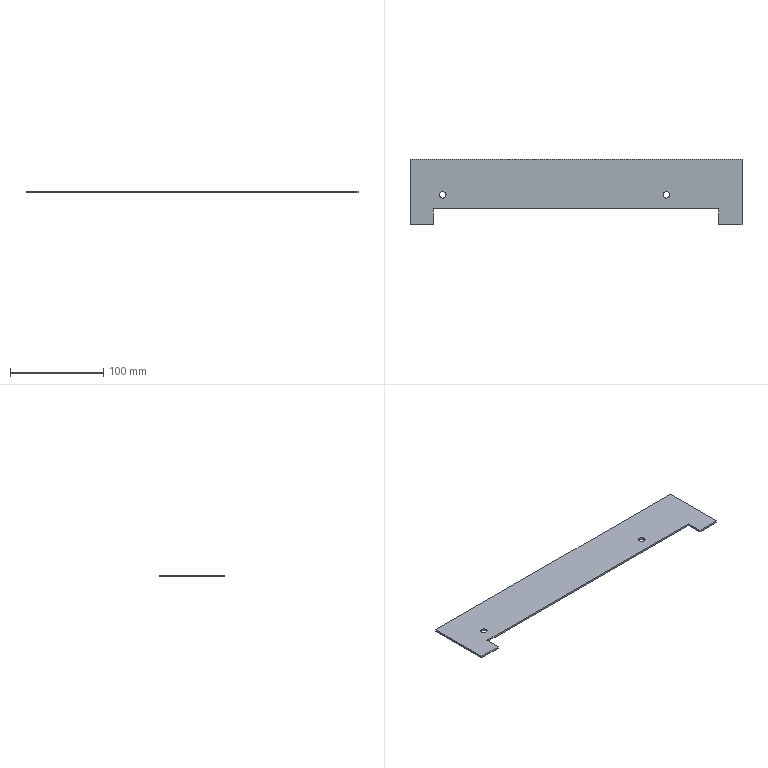Part | STEP file | xzz-004-2 | 1 solid | 14 faces | box 356 x 70 x 2 mm | volume 39282 mm3 | plane 10 | cylinder 4 | commonest cylinder face diameters 7 x4
STEP:
#1=CARTESIAN_POINT('',(-116.375,-30.,-2.));
#2=VERTEX_POINT('',#1);
#3=CARTESIAN_POINT('',(-123.375,-30.,-2.));
#4=VERTEX_POINT('',#3);
#5=CARTESIAN_POINT('',(-119.875,-30.,-2.));
#6=DIRECTION('',(0.,0.,-1.));
#7=DIRECTION('',(1.,0.,0.));
#8=AXIS2_PLACEMENT_3D('',#5,#6,#7);
#9=CIRCLE('',#8,3.5);
#10=EDGE_CURVE('',#2,#4,#9,.T.);
#11=ORIENTED_EDGE('',*,*,#10,.T.);
#12=CARTESIAN_POINT('',(-123.375,-30.,0.));
#13=VERTEX_POINT('',#12);
#14=CARTESIAN_POINT('',(-123.375,-30.,-2.));
#15=DIRECTION('',(0.,0.,1.));
#16=VECTOR('',#15,1000.);
#17=LINE('',#14,#16);
#18=EDGE_CURVE('',#4,#13,#17,.T.);
#19=ORIENTED_EDGE('',*,*,#18,.T.);
#20=CARTESIAN_POINT('',(-116.375,-30.,0.));
#21=VERTEX_POINT('',#20);
#22=CARTESIAN_POINT('',(-119.875,-30.,0.));
#23=DIRECTION('',(0.,0.,-1.));
#24=DIRECTION('',(1.,0.,0.));
#25=AXIS2_PLACEMENT_3D('',#22,#23,#24);
#26=CIRCLE('',#25,3.5);
#27=EDGE_CURVE('',#21,#13,#26,.T.);
#28=ORIENTED_EDGE('',*,*,#27,.F.);
#29=CARTESIAN_POINT('',(-116.375,-30.,-2.));
#30=DIRECTION('',(0.,0.,1.));
#31=VECTOR('',#30,1000.);
#32=LINE('',#29,#31);
#33=EDGE_CURVE('',#2,#21,#32,.T.);
#34=ORIENTED_EDGE('',*,*,#33,.F.);
#35=EDGE_LOOP('',(#11,#19,#28,#34));
#36=FACE_OUTER_BOUND('',#35,.T.);
#37=CARTESIAN_POINT('',(-119.875,-30.,-2.));
#38=DIRECTION('',(0.,0.,1.));
#39=DIRECTION('',(1.,0.,0.));
#40=AXIS2_PLACEMENT_3D('',#37,#38,#39);
#41=CYLINDRICAL_SURFACE('',#40,3.5);
#42=ADVANCED_FACE('',(#36),#41,.F.);
#43=CARTESIAN_POINT('',(123.375,-30.,-2.));
#44=VERTEX_POINT('',#43);
#45=CARTESIAN_POINT('',(116.375,-30.,-2.));
#46=VERTEX_POINT('',#45);
#47=CARTESIAN_POINT('',(119.875,-30.,-2.));
#48=DIRECTION('',(0.,0.,-1.));
#49=DIRECTION('',(1.,0.,0.));
#50=AXIS2_PLACEMENT_3D('',#47,#48,#49);
#51=CIRCLE('',#50,3.5);
#52=EDGE_CURVE('',#44,#46,#51,.T.);
#53=ORIENTED_EDGE('',*,*,#52,.T.);
#54=CARTESIAN_POINT('',(116.375,-30.,0.));
#55=VERTEX_POINT('',#54);
#56=CARTESIAN_POINT('',(116.375,-30.,-2.));
#57=DIRECTION('',(0.,0.,1.));
#58=VECTOR('',#57,1000.);
#59=LINE('',#56,#58);
#60=EDGE_CURVE('',#46,#55,#59,.T.);
#61=ORIENTED_EDGE('',*,*,#60,.T.);
#62=CARTESIAN_POINT('',(123.375,-30.,0.));
#63=VERTEX_POINT('',#62);
#64=CARTESIAN_POINT('',(119.875,-30.,0.));
#65=DIRECTION('',(0.,0.,-1.));
#66=DIRECTION('',(1.,0.,0.));
#67=AXIS2_PLACEMENT_3D('',#64,#65,#66);
#68=CIRCLE('',#67,3.5);
#69=EDGE_CURVE('',#63,#55,#68,.T.);
#70=ORIENTED_EDGE('',*,*,#69,.F.);
#71=CARTESIAN_POINT('',(123.375,-30.,-2.));
#72=DIRECTION('',(0.,0.,1.));
#73=VECTOR('',#72,1000.);
#74=LINE('',#71,#73);
#75=EDGE_CURVE('',#44,#63,#74,.T.);
#76=ORIENTED_EDGE('',*,*,#75,.F.);
#77=EDGE_LOOP('',(#53,#61,#70,#76));
#78=FACE_OUTER_BOUND('',#77,.T.);
#79=CARTESIAN_POINT('',(119.875,-30.,-2.));
#80=DIRECTION('',(0.,0.,1.));
#81=DIRECTION('',(1.,0.,0.));
#82=AXIS2_PLACEMENT_3D('',#79,#80,#81);
#83=CYLINDRICAL_SURFACE('',#82,3.5);
#84=ADVANCED_FACE('',(#78),#83,.F.);
#85=CARTESIAN_POINT('',(-130.,-62.,-2.));
#86=VERTEX_POINT('',#85);
#87=CARTESIAN_POINT('',(-130.,-45.,-2.));
#88=VERTEX_POINT('',#87);
#89=CARTESIAN_POINT('',(-130.,0.,-2.));
#90=DIRECTION('',(0.,1.,0.));
#91=VECTOR('',#90,1000.);
#92=LINE('',#89,#91);
#93=EDGE_CURVE('',#86,#88,#92,.T.);
#94=ORIENTED_EDGE('',*,*,#93,.F.);
#95=CARTESIAN_POINT('',(-155.,-62.,-2.));
#96=VERTEX_POINT('',#95);
#97=CARTESIAN_POINT('',(0.,-62.,-2.));
#98=DIRECTION('',(1.,0.,0.));
#99=VECTOR('',#98,1000.);
#100=LINE('',#97,#99);
#101=EDGE_CURVE('',#96,#86,#100,.T.);
#102=ORIENTED_EDGE('',*,*,#101,.F.);
#103=CARTESIAN_POINT('',(-155.,8.,-2.));
#104=VERTEX_POINT('',#103);
#105=CARTESIAN_POINT('',(-155.,0.,-2.));
#106=DIRECTION('',(0.,-1.,0.));
#107=VECTOR('',#106,1000.);
#108=LINE('',#105,#107);
#109=EDGE_CURVE('',#104,#96,#108,.T.);
#110=ORIENTED_EDGE('',*,*,#109,.F.);
#111=CARTESIAN_POINT('',(201.,8.,-2.));
#112=VERTEX_POINT('',#111);
#113=CARTESIAN_POINT('',(0.,8.,-2.));
#114=DIRECTION('',(-1.,0.,0.));
#115=VECTOR('',#114,1000.);
#116=LINE('',#113,#115);
#117=EDGE_CURVE('',#112,#104,#116,.T.);
#118=ORIENTED_EDGE('',*,*,#117,.F.);
#119=CARTESIAN_POINT('',(201.,-62.,-2.));
#120=VERTEX_POINT('',#119);
#121=CARTESIAN_POINT('',(201.,0.,-2.));
#122=DIRECTION('',(0.,1.,0.));
#123=VECTOR('',#122,1000.);
#124=LINE('',#121,#123);
#125=EDGE_CURVE('',#120,#112,#124,.T.);
#126=ORIENTED_EDGE('',*,*,#125,.F.);
#127=CARTESIAN_POINT('',(176.,-62.,-2.));
#128=VERTEX_POINT('',#127);
#129=CARTESIAN_POINT('',(0.,-62.,-2.));
#130=DIRECTION('',(1.,0.,0.));
#131=VECTOR('',#130,1000.);
#132=LINE('',#129,#131);
#133=EDGE_CURVE('',#128,#120,#132,.T.);
#134=ORIENTED_EDGE('',*,*,#133,.F.);
#135=CARTESIAN_POINT('',(176.,-45.,-2.));
#136=VERTEX_POINT('',#135);
#137=CARTESIAN_POINT('',(176.,0.,-2.));
#138=DIRECTION('',(0.,-1.,0.));
#139=VECTOR('',#138,1000.);
#140=LINE('',#137,#139);
#141=EDGE_CURVE('',#136,#128,#140,.T.);
#142=ORIENTED_EDGE('',*,*,#141,.F.);
#143=CARTESIAN_POINT('',(0.,-45.,-2.));
#144=DIRECTION('',(1.,0.,0.));
#145=VECTOR('',#144,1000.);
#146=LINE('',#143,#145);
#147=EDGE_CURVE('',#88,#136,#146,.T.);
#148=ORIENTED_EDGE('',*,*,#147,.F.);
#149=EDGE_LOOP('',(#94,#102,#110,#118,#126,#134,#142,#148));
#150=FACE_OUTER_BOUND('',#149,.T.);
#151=ORIENTED_EDGE('',*,*,#10,.F.);
#152=CARTESIAN_POINT('',(-119.875,-30.,-2.));
#153=DIRECTION('',(0.,0.,-1.));
#154=DIRECTION('',(1.,0.,0.));
#155=AXIS2_PLACEMENT_3D('',#152,#153,#154);
#156=CIRCLE('',#155,3.5);
#157=EDGE_CURVE('',#4,#2,#156,.T.);
#158=ORIENTED_EDGE('',*,*,#157,.F.);
#159=EDGE_LOOP('',(#151,#158));
#160=FACE_BOUND('',#159,.T.);
#161=ORIENTED_EDGE('',*,*,#52,.F.);
#162=CARTESIAN_POINT('',(119.875,-30.,-2.));
#163=DIRECTION('',(0.,0.,-1.));
#164=DIRECTION('',(1.,0.,0.));
#165=AXIS2_PLACEMENT_3D('',#162,#163,#164);
#166=CIRCLE('',#165,3.5);
#167=EDGE_CURVE('',#46,#44,#166,.T.);
#168=ORIENTED_EDGE('',*,*,#167,.F.);
#169=EDGE_LOOP('',(#161,#168));
#170=FACE_BOUND('',#169,.T.);
#171=CARTESIAN_POINT('',(0.,0.,-2.));
#172=DIRECTION('',(0.,0.,1.));
#173=DIRECTION('',(1.,0.,0.));
#174=AXIS2_PLACEMENT_3D('',#171,#172,#173);
#175=PLANE('',#174);
#176=ADVANCED_FACE('',(#150,#160,#170),#175,.F.);
#177=CARTESIAN_POINT('',(-130.,-45.,0.));
#178=VERTEX_POINT('',#177);
#179=CARTESIAN_POINT('',(176.,-45.,0.));
#180=VERTEX_POINT('',#179);
#181=CARTESIAN_POINT('',(-130.,-45.,0.));
#182=DIRECTION('',(1.,0.,0.));
#183=VECTOR('',#182,1000.);
#184=LINE('',#181,#183);
#185=EDGE_CURVE('',#178,#180,#184,.T.);
#186=ORIENTED_EDGE('',*,*,#185,.F.);
#187=CARTESIAN_POINT('',(-130.,-45.,-10.));
#188=DIRECTION('',(0.,0.,1.));
#189=VECTOR('',#188,1000.);
#190=LINE('',#187,#189);
#191=EDGE_CURVE('',#88,#178,#190,.T.);
#192=ORIENTED_EDGE('',*,*,#191,.F.);
#193=ORIENTED_EDGE('',*,*,#147,.T.);
#194=CARTESIAN_POINT('',(176.,-45.,-10.));
#195=DIRECTION('',(0.,0.,-1.));
#196=VECTOR('',#195,1000.);
#197=LINE('',#194,#196);
#198=EDGE_CURVE('',#180,#136,#197,.T.);
#199=ORIENTED_EDGE('',*,*,#198,.F.);
#200=EDGE_LOOP('',(#186,#192,#193,#199));
#201=FACE_OUTER_BOUND('',#200,.T.);
#202=CARTESIAN_POINT('',(-130.,-45.,-10.));
#203=DIRECTION('',(0.,1.,0.));
#204=DIRECTION('',(0.,0.,1.));
#205=AXIS2_PLACEMENT_3D('',#202,#203,#204);
#206=PLANE('',#205);
#207=ADVANCED_FACE('',(#201),#206,.F.);
#208=CARTESIAN_POINT('',(-130.,-62.,0.));
#209=VERTEX_POINT('',#208);
#210=CARTESIAN_POINT('',(-130.,-62.,0.));
#211=DIRECTION('',(0.,1.,0.));
#212=VECTOR('',#211,1000.);
#213=LINE('',#210,#212);
#214=EDGE_CURVE('',#209,#178,#213,.T.);
#215=ORIENTED_EDGE('',*,*,#214,.F.);
#216=CARTESIAN_POINT('',(-130.,-62.,-10.));
#217=DIRECTION('',(0.,0.,1.));
#218=VECTOR('',#217,1000.);
#219=LINE('',#216,#218);
#220=EDGE_CURVE('',#86,#209,#219,.T.);
#221=ORIENTED_EDGE('',*,*,#220,.F.);
#222=ORIENTED_EDGE('',*,*,#93,.T.);
#223=ORIENTED_EDGE('',*,*,#191,.T.);
#224=EDGE_LOOP('',(#215,#221,#222,#223));
#225=FACE_OUTER_BOUND('',#224,.T.);
#226=CARTESIAN_POINT('',(-130.,-62.,-10.));
#227=DIRECTION('',(-1.,0.,0.));
#228=DIRECTION('',(0.,0.,1.));
#229=AXIS2_PLACEMENT_3D('',#226,#227,#228);
#230=PLANE('',#229);
#231=ADVANCED_FACE('',(#225),#230,.F.);
#232=CARTESIAN_POINT('',(-155.,-62.,0.));
#233=VERTEX_POINT('',#232);
#234=CARTESIAN_POINT('',(-155.,-62.,-2.));
#235=DIRECTION('',(0.,0.,-1.));
#236=VECTOR('',#235,1000.);
#237=LINE('',#234,#236);
#238=EDGE_CURVE('',#233,#96,#237,.T.);
#239=ORIENTED_EDGE('',*,*,#238,.T.);
#240=ORIENTED_EDGE('',*,*,#101,.T.);
#241=ORIENTED_EDGE('',*,*,#220,.T.);
#242=CARTESIAN_POINT('',(-155.,-62.,0.));
#243=DIRECTION('',(-1.,0.,0.));
#244=VECTOR('',#243,1000.);
#245=LINE('',#242,#244);
#246=EDGE_CURVE('',#209,#233,#245,.T.);
#247=ORIENTED_EDGE('',*,*,#246,.T.);
#248=EDGE_LOOP('',(#239,#240,#241,#247));
#249=FACE_OUTER_BOUND('',#248,.T.);
#250=CARTESIAN_POINT('',(-155.,-62.,-2.));
#251=DIRECTION('',(0.,-1.,0.));
#252=DIRECTION('',(1.,0.,0.));
#253=AXIS2_PLACEMENT_3D('',#250,#251,#252);
#254=PLANE('',#253);
#255=ADVANCED_FACE('',(#249),#254,.T.);
#256=ORIENTED_EDGE('',*,*,#109,.T.);
#257=ORIENTED_EDGE('',*,*,#238,.F.);
#258=CARTESIAN_POINT('',(-155.,8.,0.));
#259=VERTEX_POINT('',#258);
#260=CARTESIAN_POINT('',(-155.,8.,0.));
#261=DIRECTION('',(0.,1.,0.));
#262=VECTOR('',#261,1000.);
#263=LINE('',#260,#262);
#264=EDGE_CURVE('',#233,#259,#263,.T.);
#265=ORIENTED_EDGE('',*,*,#264,.T.);
#266=CARTESIAN_POINT('',(-155.,8.,-2.));
#267=DIRECTION('',(0.,0.,-1.));
#268=VECTOR('',#267,1000.);
#269=LINE('',#266,#268);
#270=EDGE_CURVE('',#259,#104,#269,.T.);
#271=ORIENTED_EDGE('',*,*,#270,.T.);
#272=EDGE_LOOP('',(#256,#257,#265,#271));
#273=FACE_OUTER_BOUND('',#272,.T.);
#274=CARTESIAN_POINT('',(-155.,8.,-2.));
#275=DIRECTION('',(-1.,0.,0.));
#276=DIRECTION('',(0.,0.,1.));
#277=AXIS2_PLACEMENT_3D('',#274,#275,#276);
#278=PLANE('',#277);
#279=ADVANCED_FACE('',(#273),#278,.T.);
#280=ORIENTED_EDGE('',*,*,#117,.T.);
#281=ORIENTED_EDGE('',*,*,#270,.F.);
#282=CARTESIAN_POINT('',(201.,8.,0.));
#283=VERTEX_POINT('',#282);
#284=CARTESIAN_POINT('',(-155.,8.,0.));
#285=DIRECTION('',(1.,0.,0.));
#286=VECTOR('',#285,1000.);
#287=LINE('',#284,#286);
#288=EDGE_CURVE('',#259,#283,#287,.T.);
#289=ORIENTED_EDGE('',*,*,#288,.T.);
#290=CARTESIAN_POINT('',(201.,8.,-2.));
#291=DIRECTION('',(0.,0.,-1.));
#292=VECTOR('',#291,1000.);
#293=LINE('',#290,#292);
#294=EDGE_CURVE('',#283,#112,#293,.T.);
#295=ORIENTED_EDGE('',*,*,#294,.T.);
#296=EDGE_LOOP('',(#280,#281,#289,#295));
#297=FACE_OUTER_BOUND('',#296,.T.);
#298=CARTESIAN_POINT('',(-155.,8.,-2.));
#299=DIRECTION('',(0.,1.,0.));
#300=DIRECTION('',(0.,0.,1.));
#301=AXIS2_PLACEMENT_3D('',#298,#299,#300);
#302=PLANE('',#301);
#303=ADVANCED_FACE('',(#297),#302,.T.);
#304=ORIENTED_EDGE('',*,*,#125,.T.);
#305=ORIENTED_EDGE('',*,*,#294,.F.);
#306=CARTESIAN_POINT('',(201.,-62.,0.));
#307=VERTEX_POINT('',#306);
#308=CARTESIAN_POINT('',(201.,8.,0.));
#309=DIRECTION('',(0.,-1.,0.));
#310=VECTOR('',#309,1000.);
#311=LINE('',#308,#310);
#312=EDGE_CURVE('',#283,#307,#311,.T.);
#313=ORIENTED_EDGE('',*,*,#312,.T.);
#314=CARTESIAN_POINT('',(201.,-62.,-2.));
#315=DIRECTION('',(0.,0.,-1.));
#316=VECTOR('',#315,1000.);
#317=LINE('',#314,#316);
#318=EDGE_CURVE('',#307,#120,#317,.T.);
#319=ORIENTED_EDGE('',*,*,#318,.T.);
#320=EDGE_LOOP('',(#304,#305,#313,#319));
#321=FACE_OUTER_BOUND('',#320,.T.);
#322=CARTESIAN_POINT('',(201.,8.,-2.));
#323=DIRECTION('',(1.,0.,0.));
#324=DIRECTION('',(0.,1.,0.));
#325=AXIS2_PLACEMENT_3D('',#322,#323,#324);
#326=PLANE('',#325);
#327=ADVANCED_FACE('',(#321),#326,.T.);
#328=ORIENTED_EDGE('',*,*,#318,.F.);
#329=CARTESIAN_POINT('',(176.,-62.,0.));
#330=VERTEX_POINT('',#329);
#331=CARTESIAN_POINT('',(-155.,-62.,0.));
#332=DIRECTION('',(-1.,0.,0.));
#333=VECTOR('',#332,1000.);
#334=LINE('',#331,#333);
#335=EDGE_CURVE('',#307,#330,#334,.T.);
#336=ORIENTED_EDGE('',*,*,#335,.T.);
#337=CARTESIAN_POINT('',(176.,-62.,-2.));
#338=DIRECTION('',(0.,0.,-1.));
#339=VECTOR('',#338,1000.);
#340=LINE('',#337,#339);
#341=EDGE_CURVE('',#330,#128,#340,.T.);
#342=ORIENTED_EDGE('',*,*,#341,.T.);
#343=ORIENTED_EDGE('',*,*,#133,.T.);
#344=EDGE_LOOP('',(#328,#336,#342,#343));
#345=FACE_OUTER_BOUND('',#344,.T.);
#346=CARTESIAN_POINT('',(-155.,-62.,-2.));
#347=DIRECTION('',(0.,-1.,0.));
#348=DIRECTION('',(1.,0.,0.));
#349=AXIS2_PLACEMENT_3D('',#346,#347,#348);
#350=PLANE('',#349);
#351=ADVANCED_FACE('',(#345),#350,.T.);
#352=CARTESIAN_POINT('',(176.,-62.,0.));
#353=DIRECTION('',(0.,-1.,0.));
#354=VECTOR('',#353,1000.);
#355=LINE('',#352,#354);
#356=EDGE_CURVE('',#180,#330,#355,.T.);
#357=ORIENTED_EDGE('',*,*,#356,.F.);
#358=ORIENTED_EDGE('',*,*,#198,.T.);
#359=ORIENTED_EDGE('',*,*,#141,.T.);
#360=ORIENTED_EDGE('',*,*,#341,.F.);
#361=EDGE_LOOP('',(#357,#358,#359,#360));
#362=FACE_OUTER_BOUND('',#361,.T.);
#363=CARTESIAN_POINT('',(176.,-62.,-10.));
#364=DIRECTION('',(1.,0.,0.));
#365=DIRECTION('',(0.,0.,-1.));
#366=AXIS2_PLACEMENT_3D('',#363,#364,#365);
#367=PLANE('',#366);
#368=ADVANCED_FACE('',(#362),#367,.F.);
#369=ORIENTED_EDGE('',*,*,#18,.F.);
#370=ORIENTED_EDGE('',*,*,#157,.T.);
#371=ORIENTED_EDGE('',*,*,#33,.T.);
#372=CARTESIAN_POINT('',(-119.875,-30.,0.));
#373=DIRECTION('',(0.,0.,-1.));
#374=DIRECTION('',(1.,0.,0.));
#375=AXIS2_PLACEMENT_3D('',#372,#373,#374);
#376=CIRCLE('',#375,3.5);
#377=EDGE_CURVE('',#13,#21,#376,.T.);
#378=ORIENTED_EDGE('',*,*,#377,.F.);
#379=EDGE_LOOP('',(#369,#370,#371,#378));
#380=FACE_OUTER_BOUND('',#379,.T.);
#381=CARTESIAN_POINT('',(-119.875,-30.,-2.));
#382=DIRECTION('',(0.,0.,1.));
#383=DIRECTION('',(1.,0.,0.));
#384=AXIS2_PLACEMENT_3D('',#381,#382,#383);
#385=CYLINDRICAL_SURFACE('',#384,3.5);
#386=ADVANCED_FACE('',(#380),#385,.F.);
#387=ORIENTED_EDGE('',*,*,#60,.F.);
#388=ORIENTED_EDGE('',*,*,#167,.T.);
#389=ORIENTED_EDGE('',*,*,#75,.T.);
#390=CARTESIAN_POINT('',(119.875,-30.,0.));
#391=DIRECTION('',(0.,0.,-1.));
#392=DIRECTION('',(1.,0.,0.));
#393=AXIS2_PLACEMENT_3D('',#390,#391,#392);
#394=CIRCLE('',#393,3.5);
#395=EDGE_CURVE('',#55,#63,#394,.T.);
#396=ORIENTED_EDGE('',*,*,#395,.F.);
#397=EDGE_LOOP('',(#387,#388,#389,#396));
#398=FACE_OUTER_BOUND('',#397,.T.);
#399=CARTESIAN_POINT('',(119.875,-30.,-2.));
#400=DIRECTION('',(0.,0.,1.));
#401=DIRECTION('',(1.,0.,0.));
#402=AXIS2_PLACEMENT_3D('',#399,#400,#401);
#403=CYLINDRICAL_SURFACE('',#402,3.5);
#404=ADVANCED_FACE('',(#398),#403,.F.);
#405=ORIENTED_EDGE('',*,*,#27,.T.);
#406=ORIENTED_EDGE('',*,*,#377,.T.);
#407=EDGE_LOOP('',(#405,#406));
#408=FACE_BOUND('',#407,.T.);
#409=ORIENTED_EDGE('',*,*,#69,.T.);
#410=ORIENTED_EDGE('',*,*,#395,.T.);
#411=EDGE_LOOP('',(#409,#410));
#412=FACE_BOUND('',#411,.T.);
#413=ORIENTED_EDGE('',*,*,#264,.F.);
#414=ORIENTED_EDGE('',*,*,#246,.F.);
#415=ORIENTED_EDGE('',*,*,#214,.T.);
#416=ORIENTED_EDGE('',*,*,#185,.T.);
#417=ORIENTED_EDGE('',*,*,#356,.T.);
#418=ORIENTED_EDGE('',*,*,#335,.F.);
#419=ORIENTED_EDGE('',*,*,#312,.F.);
#420=ORIENTED_EDGE('',*,*,#288,.F.);
#421=EDGE_LOOP('',(#413,#414,#415,#416,#417,#418,#419,#420));
#422=FACE_OUTER_BOUND('',#421,.T.);
#423=CARTESIAN_POINT('',(0.,0.,0.));
#424=DIRECTION('',(0.,0.,1.));
#425=DIRECTION('',(1.,0.,0.));
#426=AXIS2_PLACEMENT_3D('',#423,#424,#425);
#427=PLANE('',#426);
#428=ADVANCED_FACE('',(#408,#412,#422),#427,.T.);
#429=CLOSED_SHELL('',(#42,#84,#176,#207,#231,#255,#279,#303,#327,#351,#368,#386,#404,#428));
#430=MANIFOLD_SOLID_BREP('',#429);
#431=CARTESIAN_POINT('',(0.,0.,0.));
#432=DIRECTION('',(0.,0.,1.));
#433=DIRECTION('',(1.,0.,0.));
#434=AXIS2_PLACEMENT_3D('',#431,#432,#433);
#435=(LENGTH_UNIT()NAMED_UNIT(*)SI_UNIT(.MILLI.,.METRE.));
#436=UNCERTAINTY_MEASURE_WITH_UNIT(LENGTH_MEASURE(0.00001),#435,'','');
#437=(NAMED_UNIT(*)PLANE_ANGLE_UNIT()SI_UNIT($,.RADIAN.));
#438=(NAMED_UNIT(*)SI_UNIT($,.STERADIAN.)SOLID_ANGLE_UNIT());
#439=(GEOMETRIC_REPRESENTATION_CONTEXT(3)GLOBAL_UNCERTAINTY_ASSIGNED_CONTEXT((#436))GLOBAL_UNIT_ASSIGNED_CONTEXT((#435,#437,#438))REPRESENTATION_CONTEXT('',''));
#440=ADVANCED_BREP_SHAPE_REPRESENTATION('',(#430,#434),#439);